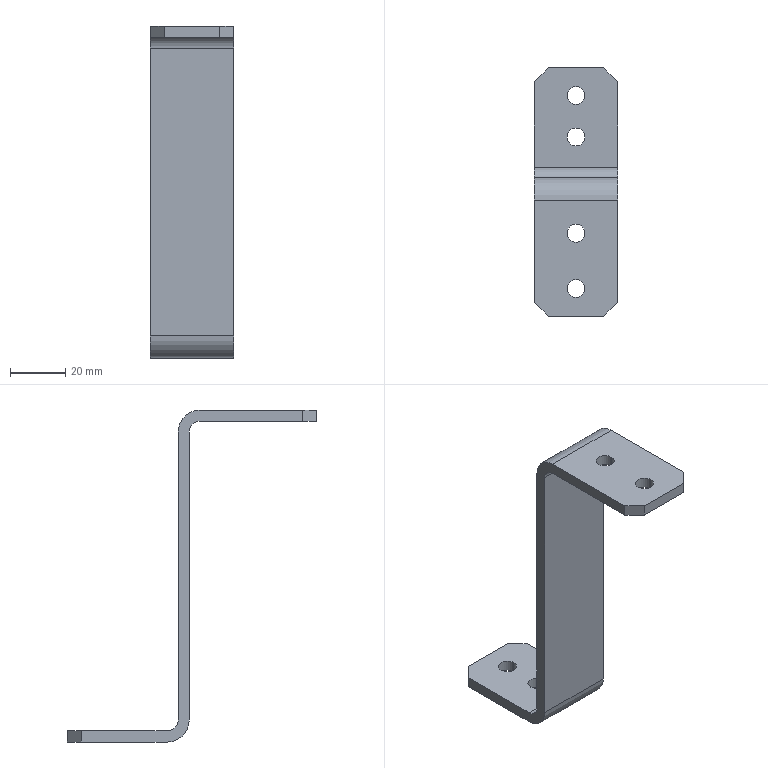Part | SolidWorks | features MBimport 1 | 1 solid | 26 faces | box 30 x 90 x 120 mm | volume 23371 mm3 | plane 14 | cylinder 12 | commonest cylinder face diameters 6.5 x8 8 x2 16 x2
STEP:
#1=CARTESIAN_POINT('',(0.,85.,-109.867));
#2=VERTEX_POINT('',#1);
#3=CARTESIAN_POINT('',(5.,90.,-109.867));
#4=VERTEX_POINT('',#3);
#5=CARTESIAN_POINT('',(5.,90.,-109.867));
#6=DIRECTION('',(0.7071,0.7071,0.));
#7=VECTOR('',#6,1000.);
#8=LINE('',#5,#7);
#9=EDGE_CURVE('',#2,#4,#8,.T.);
#10=ORIENTED_EDGE('',*,*,#9,.F.);
#11=CARTESIAN_POINT('',(0.,85.,-105.867));
#12=VERTEX_POINT('',#11);
#13=CARTESIAN_POINT('',(0.,85.,-109.867));
#14=DIRECTION('',(0.,0.,-1.));
#15=VECTOR('',#14,1000.);
#16=LINE('',#13,#15);
#17=EDGE_CURVE('',#12,#2,#16,.T.);
#18=ORIENTED_EDGE('',*,*,#17,.F.);
#19=CARTESIAN_POINT('',(5.,90.,-105.867));
#20=VERTEX_POINT('',#19);
#21=CARTESIAN_POINT('',(5.,90.,-105.867));
#22=DIRECTION('',(-0.7071,-0.7071,0.));
#23=VECTOR('',#22,1000.);
#24=LINE('',#21,#23);
#25=EDGE_CURVE('',#20,#12,#24,.T.);
#26=ORIENTED_EDGE('',*,*,#25,.F.);
#27=CARTESIAN_POINT('',(5.,90.,-105.867));
#28=DIRECTION('',(0.,0.,1.));
#29=VECTOR('',#28,1000.);
#30=LINE('',#27,#29);
#31=EDGE_CURVE('',#4,#20,#30,.T.);
#32=ORIENTED_EDGE('',*,*,#31,.F.);
#33=EDGE_LOOP('',(#10,#18,#26,#32));
#34=FACE_OUTER_BOUND('',#33,.T.);
#35=CARTESIAN_POINT('',(5.,90.,-105.867));
#36=DIRECTION('',(-0.7071,0.7071,0.));
#37=DIRECTION('',(0.,0.,1.));
#38=AXIS2_PLACEMENT_3D('',#35,#36,#37);
#39=PLANE('',#38);
#40=ADVANCED_FACE('',(#34),#39,.T.);
#41=CARTESIAN_POINT('',(25.,90.,-109.867));
#42=VERTEX_POINT('',#41);
#43=CARTESIAN_POINT('',(30.,85.,-109.867));
#44=VERTEX_POINT('',#43);
#45=CARTESIAN_POINT('',(30.,85.,-109.867));
#46=DIRECTION('',(0.7071,-0.7071,0.));
#47=VECTOR('',#46,1000.);
#48=LINE('',#45,#47);
#49=EDGE_CURVE('',#42,#44,#48,.T.);
#50=ORIENTED_EDGE('',*,*,#49,.F.);
#51=CARTESIAN_POINT('',(25.,90.,-105.867));
#52=VERTEX_POINT('',#51);
#53=CARTESIAN_POINT('',(25.,90.,-105.867));
#54=DIRECTION('',(0.,0.,-1.));
#55=VECTOR('',#54,1000.);
#56=LINE('',#53,#55);
#57=EDGE_CURVE('',#52,#42,#56,.T.);
#58=ORIENTED_EDGE('',*,*,#57,.F.);
#59=CARTESIAN_POINT('',(30.,85.,-105.867));
#60=VERTEX_POINT('',#59);
#61=CARTESIAN_POINT('',(30.,85.,-105.867));
#62=DIRECTION('',(-0.7071,0.7071,0.));
#63=VECTOR('',#62,1000.);
#64=LINE('',#61,#63);
#65=EDGE_CURVE('',#60,#52,#64,.T.);
#66=ORIENTED_EDGE('',*,*,#65,.F.);
#67=CARTESIAN_POINT('',(30.,85.,2.133));
#68=DIRECTION('',(0.,0.,1.));
#69=VECTOR('',#68,1000.);
#70=LINE('',#67,#69);
#71=EDGE_CURVE('',#44,#60,#70,.T.);
#72=ORIENTED_EDGE('',*,*,#71,.F.);
#73=EDGE_LOOP('',(#50,#58,#66,#72));
#74=FACE_OUTER_BOUND('',#73,.T.);
#75=CARTESIAN_POINT('',(30.,85.,2.133));
#76=DIRECTION('',(-0.7071,-0.7071,0.));
#77=DIRECTION('',(-0.7071,0.7071,0.));
#78=AXIS2_PLACEMENT_3D('',#75,#76,#77);
#79=PLANE('',#78);
#80=ADVANCED_FACE('',(#74),#79,.F.);
#81=CARTESIAN_POINT('',(25.,0.,10.133));
#82=VERTEX_POINT('',#81);
#83=CARTESIAN_POINT('',(30.,5.,10.133));
#84=VERTEX_POINT('',#83);
#85=CARTESIAN_POINT('',(30.,5.,10.133));
#86=DIRECTION('',(0.7071,0.7071,0.));
#87=VECTOR('',#86,1000.);
#88=LINE('',#85,#87);
#89=EDGE_CURVE('',#82,#84,#88,.T.);
#90=ORIENTED_EDGE('',*,*,#89,.F.);
#91=CARTESIAN_POINT('',(25.,0.,6.133));
#92=VERTEX_POINT('',#91);
#93=CARTESIAN_POINT('',(25.,0.,6.133));
#94=DIRECTION('',(0.,0.,1.));
#95=VECTOR('',#94,1000.);
#96=LINE('',#93,#95);
#97=EDGE_CURVE('',#92,#82,#96,.T.);
#98=ORIENTED_EDGE('',*,*,#97,.F.);
#99=CARTESIAN_POINT('',(30.,5.,6.133));
#100=VERTEX_POINT('',#99);
#101=CARTESIAN_POINT('',(30.,5.,6.133));
#102=DIRECTION('',(-0.7071,-0.7071,0.));
#103=VECTOR('',#102,1000.);
#104=LINE('',#101,#103);
#105=EDGE_CURVE('',#100,#92,#104,.T.);
#106=ORIENTED_EDGE('',*,*,#105,.F.);
#107=CARTESIAN_POINT('',(30.,5.,2.133));
#108=DIRECTION('',(0.,0.,-1.));
#109=VECTOR('',#108,1000.);
#110=LINE('',#107,#109);
#111=EDGE_CURVE('',#84,#100,#110,.T.);
#112=ORIENTED_EDGE('',*,*,#111,.F.);
#113=EDGE_LOOP('',(#90,#98,#106,#112));
#114=FACE_OUTER_BOUND('',#113,.T.);
#115=CARTESIAN_POINT('',(30.,5.,2.133));
#116=DIRECTION('',(-0.7071,0.7071,0.));
#117=DIRECTION('',(0.,0.,1.));
#118=AXIS2_PLACEMENT_3D('',#115,#116,#117);
#119=PLANE('',#118);
#120=ADVANCED_FACE('',(#114),#119,.F.);
#121=CARTESIAN_POINT('',(0.,5.,10.133));
#122=VERTEX_POINT('',#121);
#123=CARTESIAN_POINT('',(5.,0.,10.133));
#124=VERTEX_POINT('',#123);
#125=CARTESIAN_POINT('',(5.,0.,10.133));
#126=DIRECTION('',(0.7071,-0.7071,0.));
#127=VECTOR('',#126,1000.);
#128=LINE('',#125,#127);
#129=EDGE_CURVE('',#122,#124,#128,.T.);
#130=ORIENTED_EDGE('',*,*,#129,.F.);
#131=CARTESIAN_POINT('',(0.,5.,6.133));
#132=VERTEX_POINT('',#131);
#133=CARTESIAN_POINT('',(0.,5.,10.133));
#134=DIRECTION('',(0.,0.,1.));
#135=VECTOR('',#134,1000.);
#136=LINE('',#133,#135);
#137=EDGE_CURVE('',#132,#122,#136,.T.);
#138=ORIENTED_EDGE('',*,*,#137,.F.);
#139=CARTESIAN_POINT('',(5.,0.,6.133));
#140=VERTEX_POINT('',#139);
#141=CARTESIAN_POINT('',(5.,0.,6.133));
#142=DIRECTION('',(-0.7071,0.7071,0.));
#143=VECTOR('',#142,1000.);
#144=LINE('',#141,#143);
#145=EDGE_CURVE('',#140,#132,#144,.T.);
#146=ORIENTED_EDGE('',*,*,#145,.F.);
#147=CARTESIAN_POINT('',(5.,0.,6.133));
#148=DIRECTION('',(0.,0.,-1.));
#149=VECTOR('',#148,1000.);
#150=LINE('',#147,#149);
#151=EDGE_CURVE('',#124,#140,#150,.T.);
#152=ORIENTED_EDGE('',*,*,#151,.F.);
#153=EDGE_LOOP('',(#130,#138,#146,#152));
#154=FACE_OUTER_BOUND('',#153,.T.);
#155=CARTESIAN_POINT('',(5.,0.,6.133));
#156=DIRECTION('',(-0.7071,-0.7071,0.));
#157=DIRECTION('',(-0.7071,0.7071,0.));
#158=AXIS2_PLACEMENT_3D('',#155,#156,#157);
#159=PLANE('',#158);
#160=ADVANCED_FACE('',(#154),#159,.T.);
#161=CARTESIAN_POINT('',(11.75,30.,6.133));
#162=VERTEX_POINT('',#161);
#163=CARTESIAN_POINT('',(11.75,30.,10.133));
#164=VERTEX_POINT('',#163);
#165=CARTESIAN_POINT('',(11.75,30.,-19.867));
#166=DIRECTION('',(0.,0.,1.));
#167=VECTOR('',#166,1000.);
#168=LINE('',#165,#167);
#169=EDGE_CURVE('',#162,#164,#168,.T.);
#170=ORIENTED_EDGE('',*,*,#169,.F.);
#171=CARTESIAN_POINT('',(18.25,30.,6.133));
#172=VERTEX_POINT('',#171);
#173=CARTESIAN_POINT('',(15.,30.,6.133));
#174=DIRECTION('',(0.,0.,1.));
#175=DIRECTION('',(0.,-1.,0.));
#176=AXIS2_PLACEMENT_3D('',#173,#174,#175);
#177=CIRCLE('',#176,3.25);
#178=EDGE_CURVE('',#172,#162,#177,.T.);
#179=ORIENTED_EDGE('',*,*,#178,.F.);
#180=CARTESIAN_POINT('',(18.25,30.,10.133));
#181=VERTEX_POINT('',#180);
#182=CARTESIAN_POINT('',(18.25,30.,-19.867));
#183=DIRECTION('',(0.,0.,1.));
#184=VECTOR('',#183,1000.);
#185=LINE('',#182,#184);
#186=EDGE_CURVE('',#172,#181,#185,.T.);
#187=ORIENTED_EDGE('',*,*,#186,.T.);
#188=CARTESIAN_POINT('',(15.,30.,10.133));
#189=DIRECTION('',(0.,0.,1.));
#190=DIRECTION('',(1.,0.,0.));
#191=AXIS2_PLACEMENT_3D('',#188,#189,#190);
#192=CIRCLE('',#191,3.25);
#193=EDGE_CURVE('',#181,#164,#192,.T.);
#194=ORIENTED_EDGE('',*,*,#193,.T.);
#195=EDGE_LOOP('',(#170,#179,#187,#194));
#196=FACE_OUTER_BOUND('',#195,.T.);
#197=CARTESIAN_POINT('',(15.,30.,-19.867));
#198=DIRECTION('',(0.,0.,1.));
#199=DIRECTION('',(1.,0.,0.));
#200=AXIS2_PLACEMENT_3D('',#197,#198,#199);
#201=CYLINDRICAL_SURFACE('',#200,3.25);
#202=ADVANCED_FACE('',(#196),#201,.F.);
#203=CARTESIAN_POINT('',(11.75,10.,6.133));
#204=VERTEX_POINT('',#203);
#205=CARTESIAN_POINT('',(11.75,10.,10.133));
#206=VERTEX_POINT('',#205);
#207=CARTESIAN_POINT('',(11.75,10.,-19.867));
#208=DIRECTION('',(0.,0.,1.));
#209=VECTOR('',#208,1000.);
#210=LINE('',#207,#209);
#211=EDGE_CURVE('',#204,#206,#210,.T.);
#212=ORIENTED_EDGE('',*,*,#211,.F.);
#213=CARTESIAN_POINT('',(18.25,10.,6.133));
#214=VERTEX_POINT('',#213);
#215=CARTESIAN_POINT('',(15.,10.,6.133));
#216=DIRECTION('',(0.,0.,1.));
#217=DIRECTION('',(0.,-1.,0.));
#218=AXIS2_PLACEMENT_3D('',#215,#216,#217);
#219=CIRCLE('',#218,3.25);
#220=EDGE_CURVE('',#214,#204,#219,.T.);
#221=ORIENTED_EDGE('',*,*,#220,.F.);
#222=CARTESIAN_POINT('',(18.25,10.,10.133));
#223=VERTEX_POINT('',#222);
#224=CARTESIAN_POINT('',(18.25,10.,-19.867));
#225=DIRECTION('',(0.,0.,1.));
#226=VECTOR('',#225,1000.);
#227=LINE('',#224,#226);
#228=EDGE_CURVE('',#214,#223,#227,.T.);
#229=ORIENTED_EDGE('',*,*,#228,.T.);
#230=CARTESIAN_POINT('',(15.,10.,10.133));
#231=DIRECTION('',(0.,0.,1.));
#232=DIRECTION('',(1.,0.,0.));
#233=AXIS2_PLACEMENT_3D('',#230,#231,#232);
#234=CIRCLE('',#233,3.25);
#235=EDGE_CURVE('',#223,#206,#234,.T.);
#236=ORIENTED_EDGE('',*,*,#235,.T.);
#237=EDGE_LOOP('',(#212,#221,#229,#236));
#238=FACE_OUTER_BOUND('',#237,.T.);
#239=CARTESIAN_POINT('',(15.,10.,-19.867));
#240=DIRECTION('',(0.,0.,1.));
#241=DIRECTION('',(1.,0.,0.));
#242=AXIS2_PLACEMENT_3D('',#239,#240,#241);
#243=CYLINDRICAL_SURFACE('',#242,3.25);
#244=ADVANCED_FACE('',(#238),#243,.F.);
#245=CARTESIAN_POINT('',(11.75,80.,-109.867));
#246=VERTEX_POINT('',#245);
#247=CARTESIAN_POINT('',(11.75,80.,-105.867));
#248=VERTEX_POINT('',#247);
#249=CARTESIAN_POINT('',(11.75,80.,-135.867));
#250=DIRECTION('',(0.,0.,1.));
#251=VECTOR('',#250,1000.);
#252=LINE('',#249,#251);
#253=EDGE_CURVE('',#246,#248,#252,.T.);
#254=ORIENTED_EDGE('',*,*,#253,.F.);
#255=CARTESIAN_POINT('',(18.25,80.,-109.867));
#256=VERTEX_POINT('',#255);
#257=CARTESIAN_POINT('',(15.,80.,-109.867));
#258=DIRECTION('',(0.,0.,1.));
#259=DIRECTION('',(0.,-1.,0.));
#260=AXIS2_PLACEMENT_3D('',#257,#258,#259);
#261=CIRCLE('',#260,3.25);
#262=EDGE_CURVE('',#256,#246,#261,.T.);
#263=ORIENTED_EDGE('',*,*,#262,.F.);
#264=CARTESIAN_POINT('',(18.25,80.,-105.867));
#265=VERTEX_POINT('',#264);
#266=CARTESIAN_POINT('',(18.25,80.,-135.867));
#267=DIRECTION('',(0.,0.,1.));
#268=VECTOR('',#267,1000.);
#269=LINE('',#266,#268);
#270=EDGE_CURVE('',#256,#265,#269,.T.);
#271=ORIENTED_EDGE('',*,*,#270,.T.);
#272=CARTESIAN_POINT('',(15.,80.,-105.867));
#273=DIRECTION('',(0.,0.,1.));
#274=DIRECTION('',(1.,0.,0.));
#275=AXIS2_PLACEMENT_3D('',#272,#273,#274);
#276=CIRCLE('',#275,3.25);
#277=EDGE_CURVE('',#265,#248,#276,.T.);
#278=ORIENTED_EDGE('',*,*,#277,.T.);
#279=EDGE_LOOP('',(#254,#263,#271,#278));
#280=FACE_OUTER_BOUND('',#279,.T.);
#281=CARTESIAN_POINT('',(15.,80.,-135.867));
#282=DIRECTION('',(0.,0.,1.));
#283=DIRECTION('',(1.,0.,0.));
#284=AXIS2_PLACEMENT_3D('',#281,#282,#283);
#285=CYLINDRICAL_SURFACE('',#284,3.25);
#286=ADVANCED_FACE('',(#280),#285,.F.);
#287=CARTESIAN_POINT('',(11.75,65.,-109.867));
#288=VERTEX_POINT('',#287);
#289=CARTESIAN_POINT('',(11.75,65.,-105.867));
#290=VERTEX_POINT('',#289);
#291=CARTESIAN_POINT('',(11.75,65.,-135.867));
#292=DIRECTION('',(0.,0.,1.));
#293=VECTOR('',#292,1000.);
#294=LINE('',#291,#293);
#295=EDGE_CURVE('',#288,#290,#294,.T.);
#296=ORIENTED_EDGE('',*,*,#295,.F.);
#297=CARTESIAN_POINT('',(18.25,65.,-109.867));
#298=VERTEX_POINT('',#297);
#299=CARTESIAN_POINT('',(15.,65.,-109.867));
#300=DIRECTION('',(0.,0.,1.));
#301=DIRECTION('',(0.,-1.,0.));
#302=AXIS2_PLACEMENT_3D('',#299,#300,#301);
#303=CIRCLE('',#302,3.25);
#304=EDGE_CURVE('',#298,#288,#303,.T.);
#305=ORIENTED_EDGE('',*,*,#304,.F.);
#306=CARTESIAN_POINT('',(18.25,65.,-105.867));
#307=VERTEX_POINT('',#306);
#308=CARTESIAN_POINT('',(18.25,65.,-135.867));
#309=DIRECTION('',(0.,0.,1.));
#310=VECTOR('',#309,1000.);
#311=LINE('',#308,#310);
#312=EDGE_CURVE('',#298,#307,#311,.T.);
#313=ORIENTED_EDGE('',*,*,#312,.T.);
#314=CARTESIAN_POINT('',(15.,65.,-105.867));
#315=DIRECTION('',(0.,0.,1.));
#316=DIRECTION('',(1.,0.,0.));
#317=AXIS2_PLACEMENT_3D('',#314,#315,#316);
#318=CIRCLE('',#317,3.25);
#319=EDGE_CURVE('',#307,#290,#318,.T.);
#320=ORIENTED_EDGE('',*,*,#319,.T.);
#321=EDGE_LOOP('',(#296,#305,#313,#320));
#322=FACE_OUTER_BOUND('',#321,.T.);
#323=CARTESIAN_POINT('',(15.,65.,-135.867));
#324=DIRECTION('',(0.,0.,1.));
#325=DIRECTION('',(1.,0.,0.));
#326=AXIS2_PLACEMENT_3D('',#323,#324,#325);
#327=CYLINDRICAL_SURFACE('',#326,3.25);
#328=ADVANCED_FACE('',(#322),#327,.F.);
#329=CARTESIAN_POINT('',(0.,42.,6.133));
#330=VERTEX_POINT('',#329);
#331=CARTESIAN_POINT('',(0.,42.,6.133));
#332=DIRECTION('',(0.,1.,0.));
#333=VECTOR('',#332,1000.);
#334=LINE('',#331,#333);
#335=EDGE_CURVE('',#132,#330,#334,.T.);
#336=ORIENTED_EDGE('',*,*,#335,.F.);
#337=ORIENTED_EDGE('',*,*,#137,.T.);
#338=CARTESIAN_POINT('',(0.,42.,10.133));
#339=VERTEX_POINT('',#338);
#340=CARTESIAN_POINT('',(0.,0.,10.133));
#341=DIRECTION('',(0.,-1.,0.));
#342=VECTOR('',#341,1000.);
#343=LINE('',#340,#342);
#344=EDGE_CURVE('',#339,#122,#343,.T.);
#345=ORIENTED_EDGE('',*,*,#344,.F.);
#346=CARTESIAN_POINT('',(0.,50.,2.133));
#347=VERTEX_POINT('',#346);
#348=CARTESIAN_POINT('',(0.,42.,2.133));
#349=DIRECTION('',(1.,0.,0.));
#350=DIRECTION('',(0.,0.,1.));
#351=AXIS2_PLACEMENT_3D('',#348,#349,#350);
#352=CIRCLE('',#351,8.);
#353=EDGE_CURVE('',#347,#339,#352,.T.);
#354=ORIENTED_EDGE('',*,*,#353,.F.);
#355=CARTESIAN_POINT('',(0.,50.,-101.867));
#356=VERTEX_POINT('',#355);
#357=CARTESIAN_POINT('',(0.,50.,2.133));
#358=DIRECTION('',(0.,0.,1.));
#359=VECTOR('',#358,1000.);
#360=LINE('',#357,#359);
#361=EDGE_CURVE('',#356,#347,#360,.T.);
#362=ORIENTED_EDGE('',*,*,#361,.F.);
#363=CARTESIAN_POINT('',(0.,54.,-105.867));
#364=VERTEX_POINT('',#363);
#365=CARTESIAN_POINT('',(0.,54.,-101.867));
#366=DIRECTION('',(-1.,0.,0.));
#367=DIRECTION('',(0.,0.,-1.));
#368=AXIS2_PLACEMENT_3D('',#365,#366,#367);
#369=CIRCLE('',#368,4.);
#370=EDGE_CURVE('',#364,#356,#369,.T.);
#371=ORIENTED_EDGE('',*,*,#370,.F.);
#372=CARTESIAN_POINT('',(0.,54.,-105.867));
#373=DIRECTION('',(0.,-1.,0.));
#374=VECTOR('',#373,1000.);
#375=LINE('',#372,#374);
#376=EDGE_CURVE('',#12,#364,#375,.T.);
#377=ORIENTED_EDGE('',*,*,#376,.F.);
#378=ORIENTED_EDGE('',*,*,#17,.T.);
#379=CARTESIAN_POINT('',(0.,54.,-109.867));
#380=VERTEX_POINT('',#379);
#381=CARTESIAN_POINT('',(0.,90.,-109.867));
#382=DIRECTION('',(0.,1.,0.));
#383=VECTOR('',#382,1000.);
#384=LINE('',#381,#383);
#385=EDGE_CURVE('',#380,#2,#384,.T.);
#386=ORIENTED_EDGE('',*,*,#385,.F.);
#387=CARTESIAN_POINT('',(0.,46.,-101.867));
#388=VERTEX_POINT('',#387);
#389=CARTESIAN_POINT('',(0.,54.,-101.867));
#390=DIRECTION('',(1.,0.,0.));
#391=DIRECTION('',(0.,0.,-1.));
#392=AXIS2_PLACEMENT_3D('',#389,#390,#391);
#393=CIRCLE('',#392,8.);
#394=EDGE_CURVE('',#388,#380,#393,.T.);
#395=ORIENTED_EDGE('',*,*,#394,.F.);
#396=CARTESIAN_POINT('',(0.,46.,2.133));
#397=VERTEX_POINT('',#396);
#398=CARTESIAN_POINT('',(0.,46.,-101.867));
#399=DIRECTION('',(0.,0.,-1.));
#400=VECTOR('',#399,1000.);
#401=LINE('',#398,#400);
#402=EDGE_CURVE('',#397,#388,#401,.T.);
#403=ORIENTED_EDGE('',*,*,#402,.F.);
#404=CARTESIAN_POINT('',(0.,42.,2.133));
#405=DIRECTION('',(-1.,0.,0.));
#406=DIRECTION('',(0.,0.,1.));
#407=AXIS2_PLACEMENT_3D('',#404,#405,#406);
#408=CIRCLE('',#407,4.);
#409=EDGE_CURVE('',#330,#397,#408,.T.);
#410=ORIENTED_EDGE('',*,*,#409,.F.);
#411=EDGE_LOOP('',(#336,#337,#345,#354,#362,#371,#377,#378,#386,#395,#403,#410));
#412=FACE_OUTER_BOUND('',#411,.T.);
#413=CARTESIAN_POINT('',(0.,42.,2.133));
#414=DIRECTION('',(-1.,0.,0.));
#415=DIRECTION('',(0.,0.,1.));
#416=AXIS2_PLACEMENT_3D('',#413,#414,#415);
#417=PLANE('',#416);
#418=ADVANCED_FACE('',(#412),#417,.T.);
#419=CARTESIAN_POINT('',(30.,42.,10.133));
#420=VERTEX_POINT('',#419);
#421=CARTESIAN_POINT('',(30.,0.,10.133));
#422=DIRECTION('',(0.,-1.,0.));
#423=VECTOR('',#422,1000.);
#424=LINE('',#421,#423);
#425=EDGE_CURVE('',#420,#84,#424,.T.);
#426=ORIENTED_EDGE('',*,*,#425,.T.);
#427=ORIENTED_EDGE('',*,*,#111,.T.);
#428=CARTESIAN_POINT('',(30.,42.,6.133));
#429=VERTEX_POINT('',#428);
#430=CARTESIAN_POINT('',(30.,42.,6.133));
#431=DIRECTION('',(0.,1.,0.));
#432=VECTOR('',#431,1000.);
#433=LINE('',#430,#432);
#434=EDGE_CURVE('',#100,#429,#433,.T.);
#435=ORIENTED_EDGE('',*,*,#434,.T.);
#436=CARTESIAN_POINT('',(30.,46.,2.133));
#437=VERTEX_POINT('',#436);
#438=CARTESIAN_POINT('',(30.,42.,2.133));
#439=DIRECTION('',(-1.,0.,0.));
#440=DIRECTION('',(0.,0.,1.));
#441=AXIS2_PLACEMENT_3D('',#438,#439,#440);
#442=CIRCLE('',#441,4.);
#443=EDGE_CURVE('',#429,#437,#442,.T.);
#444=ORIENTED_EDGE('',*,*,#443,.T.);
#445=CARTESIAN_POINT('',(30.,46.,-101.867));
#446=VERTEX_POINT('',#445);
#447=CARTESIAN_POINT('',(30.,46.,-101.867));
#448=DIRECTION('',(0.,0.,-1.));
#449=VECTOR('',#448,1000.);
#450=LINE('',#447,#449);
#451=EDGE_CURVE('',#437,#446,#450,.T.);
#452=ORIENTED_EDGE('',*,*,#451,.T.);
#453=CARTESIAN_POINT('',(30.,54.,-109.867));
#454=VERTEX_POINT('',#453);
#455=CARTESIAN_POINT('',(30.,54.,-101.867));
#456=DIRECTION('',(1.,0.,0.));
#457=DIRECTION('',(0.,0.,-1.));
#458=AXIS2_PLACEMENT_3D('',#455,#456,#457);
#459=CIRCLE('',#458,8.);
#460=EDGE_CURVE('',#446,#454,#459,.T.);
#461=ORIENTED_EDGE('',*,*,#460,.T.);
#462=CARTESIAN_POINT('',(30.,90.,-109.867));
#463=DIRECTION('',(0.,1.,0.));
#464=VECTOR('',#463,1000.);
#465=LINE('',#462,#464);
#466=EDGE_CURVE('',#454,#44,#465,.T.);
#467=ORIENTED_EDGE('',*,*,#466,.T.);
#468=ORIENTED_EDGE('',*,*,#71,.T.);
#469=CARTESIAN_POINT('',(30.,54.,-105.867));
#470=VERTEX_POINT('',#469);
#471=CARTESIAN_POINT('',(30.,54.,-105.867));
#472=DIRECTION('',(0.,-1.,0.));
#473=VECTOR('',#472,1000.);
#474=LINE('',#471,#473);
#475=EDGE_CURVE('',#60,#470,#474,.T.);
#476=ORIENTED_EDGE('',*,*,#475,.T.);
#477=CARTESIAN_POINT('',(30.,50.,-101.867));
#478=VERTEX_POINT('',#477);
#479=CARTESIAN_POINT('',(30.,54.,-101.867));
#480=DIRECTION('',(-1.,0.,0.));
#481=DIRECTION('',(0.,0.,-1.));
#482=AXIS2_PLACEMENT_3D('',#479,#480,#481);
#483=CIRCLE('',#482,4.);
#484=EDGE_CURVE('',#470,#478,#483,.T.);
#485=ORIENTED_EDGE('',*,*,#484,.T.);
#486=CARTESIAN_POINT('',(30.,50.,2.133));
#487=VERTEX_POINT('',#486);
#488=CARTESIAN_POINT('',(30.,50.,2.133));
#489=DIRECTION('',(0.,0.,1.));
#490=VECTOR('',#489,1000.);
#491=LINE('',#488,#490);
#492=EDGE_CURVE('',#478,#487,#491,.T.);
#493=ORIENTED_EDGE('',*,*,#492,.T.);
#494=CARTESIAN_POINT('',(30.,42.,2.133));
#495=DIRECTION('',(1.,0.,0.));
#496=DIRECTION('',(0.,0.,1.));
#497=AXIS2_PLACEMENT_3D('',#494,#495,#496);
#498=CIRCLE('',#497,8.);
#499=EDGE_CURVE('',#487,#420,#498,.T.);
#500=ORIENTED_EDGE('',*,*,#499,.T.);
#501=EDGE_LOOP('',(#426,#427,#435,#444,#452,#461,#467,#468,#476,#485,#493,#500));
#502=FACE_OUTER_BOUND('',#501,.T.);
#503=CARTESIAN_POINT('',(30.,42.,2.133));
#504=DIRECTION('',(-1.,0.,0.));
#505=DIRECTION('',(0.,0.,1.));
#506=AXIS2_PLACEMENT_3D('',#503,#504,#505);
#507=PLANE('',#506);
#508=ADVANCED_FACE('',(#502),#507,.F.);
#509=CARTESIAN_POINT('',(30.,0.,10.133));
#510=DIRECTION('',(-1.,0.,0.));
#511=VECTOR('',#510,1000.);
#512=LINE('',#509,#511);
#513=EDGE_CURVE('',#82,#124,#512,.T.);
#514=ORIENTED_EDGE('',*,*,#513,.T.);
#515=ORIENTED_EDGE('',*,*,#151,.T.);
#516=CARTESIAN_POINT('',(30.,0.,6.133));
#517=DIRECTION('',(-1.,0.,0.));
#518=VECTOR('',#517,1000.);
#519=LINE('',#516,#518);
#520=EDGE_CURVE('',#92,#140,#519,.T.);
#521=ORIENTED_EDGE('',*,*,#520,.F.);
#522=ORIENTED_EDGE('',*,*,#97,.T.);
#523=EDGE_LOOP('',(#514,#515,#521,#522));
#524=FACE_OUTER_BOUND('',#523,.T.);
#525=CARTESIAN_POINT('',(30.,0.,6.133));
#526=DIRECTION('',(0.,1.,0.));
#527=DIRECTION('',(1.,0.,0.));
#528=AXIS2_PLACEMENT_3D('',#525,#526,#527);
#529=PLANE('',#528);
#530=ADVANCED_FACE('',(#524),#529,.F.);
#531=ORIENTED_EDGE('',*,*,#235,.F.);
#532=CARTESIAN_POINT('',(15.,10.,10.133));
#533=DIRECTION('',(0.,0.,1.));
#534=DIRECTION('',(1.,0.,0.));
#535=AXIS2_PLACEMENT_3D('',#532,#533,#534);
#536=CIRCLE('',#535,3.25);
#537=EDGE_CURVE('',#206,#223,#536,.T.);
#538=ORIENTED_EDGE('',*,*,#537,.F.);
#539=EDGE_LOOP('',(#531,#538));
#540=FACE_BOUND('',#539,.T.);
#541=ORIENTED_EDGE('',*,*,#193,.F.);
#542=CARTESIAN_POINT('',(15.,30.,10.133));
#543=DIRECTION('',(0.,0.,1.));
#544=DIRECTION('',(1.,0.,0.));
#545=AXIS2_PLACEMENT_3D('',#542,#543,#544);
#546=CIRCLE('',#545,3.25);
#547=EDGE_CURVE('',#164,#181,#546,.T.);
#548=ORIENTED_EDGE('',*,*,#547,.F.);
#549=EDGE_LOOP('',(#541,#548));
#550=FACE_BOUND('',#549,.T.);
#551=ORIENTED_EDGE('',*,*,#344,.T.);
#552=ORIENTED_EDGE('',*,*,#129,.T.);
#553=ORIENTED_EDGE('',*,*,#513,.F.);
#554=ORIENTED_EDGE('',*,*,#89,.T.);
#555=ORIENTED_EDGE('',*,*,#425,.F.);
#556=CARTESIAN_POINT('',(30.,42.,10.133));
#557=DIRECTION('',(-1.,0.,0.));
#558=VECTOR('',#557,1000.);
#559=LINE('',#556,#558);
#560=EDGE_CURVE('',#420,#339,#559,.T.);
#561=ORIENTED_EDGE('',*,*,#560,.T.);
#562=EDGE_LOOP('',(#551,#552,#553,#554,#555,#561));
#563=FACE_OUTER_BOUND('',#562,.T.);
#564=CARTESIAN_POINT('',(30.,0.,10.133));
#565=DIRECTION('',(0.,0.,-1.));
#566=DIRECTION('',(0.,-1.,0.));
#567=AXIS2_PLACEMENT_3D('',#564,#565,#566);
#568=PLANE('',#567);
#569=ADVANCED_FACE('',(#540,#550,#563),#568,.F.);
#570=ORIENTED_EDGE('',*,*,#353,.T.);
#571=ORIENTED_EDGE('',*,*,#560,.F.);
#572=ORIENTED_EDGE('',*,*,#499,.F.);
#573=CARTESIAN_POINT('',(30.,50.,2.133));
#574=DIRECTION('',(-1.,0.,0.));
#575=VECTOR('',#574,1000.);
#576=LINE('',#573,#575);
#577=EDGE_CURVE('',#487,#347,#576,.T.);
#578=ORIENTED_EDGE('',*,*,#577,.T.);
#579=EDGE_LOOP('',(#570,#571,#572,#578));
#580=FACE_OUTER_BOUND('',#579,.T.);
#581=CARTESIAN_POINT('',(30.,42.,2.133));
#582=DIRECTION('',(-1.,0.,0.));
#583=DIRECTION('',(0.,0.,1.));
#584=AXIS2_PLACEMENT_3D('',#581,#582,#583);
#585=CYLINDRICAL_SURFACE('',#584,8.);
#586=ADVANCED_FACE('',(#580),#585,.T.);
#587=ORIENTED_EDGE('',*,*,#361,.T.);
#588=ORIENTED_EDGE('',*,*,#577,.F.);
#589=ORIENTED_EDGE('',*,*,#492,.F.);
#590=CARTESIAN_POINT('',(30.,50.,-101.867));
#591=DIRECTION('',(-1.,0.,0.));
#592=VECTOR('',#591,1000.);
#593=LINE('',#590,#592);
#594=EDGE_CURVE('',#478,#356,#593,.T.);
#595=ORIENTED_EDGE('',*,*,#594,.T.);
#596=EDGE_LOOP('',(#587,#588,#589,#595));
#597=FACE_OUTER_BOUND('',#596,.T.);
#598=CARTESIAN_POINT('',(30.,50.,2.133));
#599=DIRECTION('',(0.,-1.,0.));
#600=DIRECTION('',(0.,0.,-1.));
#601=AXIS2_PLACEMENT_3D('',#598,#599,#600);
#602=PLANE('',#601);
#603=ADVANCED_FACE('',(#597),#602,.F.);
#604=ORIENTED_EDGE('',*,*,#370,.T.);
#605=ORIENTED_EDGE('',*,*,#594,.F.);
#606=ORIENTED_EDGE('',*,*,#484,.F.);
#607=CARTESIAN_POINT('',(30.,54.,-105.867));
#608=DIRECTION('',(-1.,0.,0.));
#609=VECTOR('',#608,1000.);
#610=LINE('',#607,#609);
#611=EDGE_CURVE('',#470,#364,#610,.T.);
#612=ORIENTED_EDGE('',*,*,#611,.T.);
#613=EDGE_LOOP('',(#604,#605,#606,#612));
#614=FACE_OUTER_BOUND('',#613,.T.);
#615=CARTESIAN_POINT('',(30.,54.,-101.867));
#616=DIRECTION('',(-1.,0.,0.));
#617=DIRECTION('',(0.,0.,1.));
#618=AXIS2_PLACEMENT_3D('',#615,#616,#617);
#619=CYLINDRICAL_SURFACE('',#618,4.);
#620=ADVANCED_FACE('',(#614),#619,.F.);
#621=ORIENTED_EDGE('',*,*,#319,.F.);
#622=CARTESIAN_POINT('',(15.,65.,-105.867));
#623=DIRECTION('',(0.,0.,1.));
#624=DIRECTION('',(1.,0.,0.));
#625=AXIS2_PLACEMENT_3D('',#622,#623,#624);
#626=CIRCLE('',#625,3.25);
#627=EDGE_CURVE('',#290,#307,#626,.T.);
#628=ORIENTED_EDGE('',*,*,#627,.F.);
#629=EDGE_LOOP('',(#621,#628));
#630=FACE_BOUND('',#629,.T.);
#631=ORIENTED_EDGE('',*,*,#277,.F.);
#632=CARTESIAN_POINT('',(15.,80.,-105.867));
#633=DIRECTION('',(0.,0.,1.));
#634=DIRECTION('',(1.,0.,0.));
#635=AXIS2_PLACEMENT_3D('',#632,#633,#634);
#636=CIRCLE('',#635,3.25);
#637=EDGE_CURVE('',#248,#265,#636,.T.);
#638=ORIENTED_EDGE('',*,*,#637,.F.);
#639=EDGE_LOOP('',(#631,#638));
#640=FACE_BOUND('',#639,.T.);
#641=ORIENTED_EDGE('',*,*,#475,.F.);
#642=ORIENTED_EDGE('',*,*,#65,.T.);
#643=CARTESIAN_POINT('',(30.,90.,-105.867));
#644=DIRECTION('',(-1.,0.,0.));
#645=VECTOR('',#644,1000.);
#646=LINE('',#643,#645);
#647=EDGE_CURVE('',#52,#20,#646,.T.);
#648=ORIENTED_EDGE('',*,*,#647,.T.);
#649=ORIENTED_EDGE('',*,*,#25,.T.);
#650=ORIENTED_EDGE('',*,*,#376,.T.);
#651=ORIENTED_EDGE('',*,*,#611,.F.);
#652=EDGE_LOOP('',(#641,#642,#648,#649,#650,#651));
#653=FACE_OUTER_BOUND('',#652,.T.);
#654=CARTESIAN_POINT('',(30.,54.,-105.867));
#655=DIRECTION('',(0.,0.,-1.));
#656=DIRECTION('',(0.,-1.,0.));
#657=AXIS2_PLACEMENT_3D('',#654,#655,#656);
#658=PLANE('',#657);
#659=ADVANCED_FACE('',(#630,#640,#653),#658,.F.);
#660=ORIENTED_EDGE('',*,*,#647,.F.);
#661=ORIENTED_EDGE('',*,*,#57,.T.);
#662=CARTESIAN_POINT('',(30.,90.,-109.867));
#663=DIRECTION('',(-1.,0.,0.));
#664=VECTOR('',#663,1000.);
#665=LINE('',#662,#664);
#666=EDGE_CURVE('',#42,#4,#665,.T.);
#667=ORIENTED_EDGE('',*,*,#666,.T.);
#668=ORIENTED_EDGE('',*,*,#31,.T.);
#669=EDGE_LOOP('',(#660,#661,#667,#668));
#670=FACE_OUTER_BOUND('',#669,.T.);
#671=CARTESIAN_POINT('',(30.,90.,-105.867));
#672=DIRECTION('',(0.,-1.,0.));
#673=DIRECTION('',(0.,0.,-1.));
#674=AXIS2_PLACEMENT_3D('',#671,#672,#673);
#675=PLANE('',#674);
#676=ADVANCED_FACE('',(#670),#675,.F.);
#677=ORIENTED_EDGE('',*,*,#304,.T.);
#678=CARTESIAN_POINT('',(15.,65.,-109.867));
#679=DIRECTION('',(0.,0.,1.));
#680=DIRECTION('',(0.,-1.,0.));
#681=AXIS2_PLACEMENT_3D('',#678,#679,#680);
#682=CIRCLE('',#681,3.25);
#683=EDGE_CURVE('',#288,#298,#682,.T.);
#684=ORIENTED_EDGE('',*,*,#683,.T.);
#685=EDGE_LOOP('',(#677,#684));
#686=FACE_BOUND('',#685,.T.);
#687=ORIENTED_EDGE('',*,*,#262,.T.);
#688=CARTESIAN_POINT('',(15.,80.,-109.867));
#689=DIRECTION('',(0.,0.,1.));
#690=DIRECTION('',(0.,-1.,0.));
#691=AXIS2_PLACEMENT_3D('',#688,#689,#690);
#692=CIRCLE('',#691,3.25);
#693=EDGE_CURVE('',#246,#256,#692,.T.);
#694=ORIENTED_EDGE('',*,*,#693,.T.);
#695=EDGE_LOOP('',(#687,#694));
#696=FACE_BOUND('',#695,.T.);
#697=ORIENTED_EDGE('',*,*,#666,.F.);
#698=ORIENTED_EDGE('',*,*,#49,.T.);
#699=ORIENTED_EDGE('',*,*,#466,.F.);
#700=CARTESIAN_POINT('',(30.,54.,-109.867));
#701=DIRECTION('',(-1.,0.,0.));
#702=VECTOR('',#701,1000.);
#703=LINE('',#700,#702);
#704=EDGE_CURVE('',#454,#380,#703,.T.);
#705=ORIENTED_EDGE('',*,*,#704,.T.);
#706=ORIENTED_EDGE('',*,*,#385,.T.);
#707=ORIENTED_EDGE('',*,*,#9,.T.);
#708=EDGE_LOOP('',(#697,#698,#699,#705,#706,#707));
#709=FACE_OUTER_BOUND('',#708,.T.);
#710=CARTESIAN_POINT('',(30.,90.,-109.867));
#711=DIRECTION('',(0.,0.,1.));
#712=DIRECTION('',(0.,-1.,0.));
#713=AXIS2_PLACEMENT_3D('',#710,#711,#712);
#714=PLANE('',#713);
#715=ADVANCED_FACE('',(#686,#696,#709),#714,.F.);
#716=ORIENTED_EDGE('',*,*,#394,.T.);
#717=ORIENTED_EDGE('',*,*,#704,.F.);
#718=ORIENTED_EDGE('',*,*,#460,.F.);
#719=CARTESIAN_POINT('',(30.,46.,-101.867));
#720=DIRECTION('',(-1.,0.,0.));
#721=VECTOR('',#720,1000.);
#722=LINE('',#719,#721);
#723=EDGE_CURVE('',#446,#388,#722,.T.);
#724=ORIENTED_EDGE('',*,*,#723,.T.);
#725=EDGE_LOOP('',(#716,#717,#718,#724));
#726=FACE_OUTER_BOUND('',#725,.T.);
#727=CARTESIAN_POINT('',(30.,54.,-101.867));
#728=DIRECTION('',(-1.,0.,0.));
#729=DIRECTION('',(0.,0.,1.));
#730=AXIS2_PLACEMENT_3D('',#727,#728,#729);
#731=CYLINDRICAL_SURFACE('',#730,8.);
#732=ADVANCED_FACE('',(#726),#731,.T.);
#733=ORIENTED_EDGE('',*,*,#402,.T.);
#734=ORIENTED_EDGE('',*,*,#723,.F.);
#735=ORIENTED_EDGE('',*,*,#451,.F.);
#736=CARTESIAN_POINT('',(30.,46.,2.133));
#737=DIRECTION('',(-1.,0.,0.));
#738=VECTOR('',#737,1000.);
#739=LINE('',#736,#738);
#740=EDGE_CURVE('',#437,#397,#739,.T.);
#741=ORIENTED_EDGE('',*,*,#740,.T.);
#742=EDGE_LOOP('',(#733,#734,#735,#741));
#743=FACE_OUTER_BOUND('',#742,.T.);
#744=CARTESIAN_POINT('',(30.,46.,-101.867));
#745=DIRECTION('',(0.,1.,0.));
#746=DIRECTION('',(1.,0.,0.));
#747=AXIS2_PLACEMENT_3D('',#744,#745,#746);
#748=PLANE('',#747);
#749=ADVANCED_FACE('',(#743),#748,.F.);
#750=ORIENTED_EDGE('',*,*,#409,.T.);
#751=ORIENTED_EDGE('',*,*,#740,.F.);
#752=ORIENTED_EDGE('',*,*,#443,.F.);
#753=CARTESIAN_POINT('',(30.,42.,6.133));
#754=DIRECTION('',(-1.,0.,0.));
#755=VECTOR('',#754,1000.);
#756=LINE('',#753,#755);
#757=EDGE_CURVE('',#429,#330,#756,.T.);
#758=ORIENTED_EDGE('',*,*,#757,.T.);
#759=EDGE_LOOP('',(#750,#751,#752,#758));
#760=FACE_OUTER_BOUND('',#759,.T.);
#761=CARTESIAN_POINT('',(30.,42.,2.133));
#762=DIRECTION('',(-1.,0.,0.));
#763=DIRECTION('',(0.,0.,1.));
#764=AXIS2_PLACEMENT_3D('',#761,#762,#763);
#765=CYLINDRICAL_SURFACE('',#764,4.);
#766=ADVANCED_FACE('',(#760),#765,.F.);
#767=ORIENTED_EDGE('',*,*,#220,.T.);
#768=CARTESIAN_POINT('',(15.,10.,6.133));
#769=DIRECTION('',(0.,0.,1.));
#770=DIRECTION('',(0.,-1.,0.));
#771=AXIS2_PLACEMENT_3D('',#768,#769,#770);
#772=CIRCLE('',#771,3.25);
#773=EDGE_CURVE('',#204,#214,#772,.T.);
#774=ORIENTED_EDGE('',*,*,#773,.T.);
#775=EDGE_LOOP('',(#767,#774));
#776=FACE_BOUND('',#775,.T.);
#777=ORIENTED_EDGE('',*,*,#178,.T.);
#778=CARTESIAN_POINT('',(15.,30.,6.133));
#779=DIRECTION('',(0.,0.,1.));
#780=DIRECTION('',(0.,-1.,0.));
#781=AXIS2_PLACEMENT_3D('',#778,#779,#780);
#782=CIRCLE('',#781,3.25);
#783=EDGE_CURVE('',#162,#172,#782,.T.);
#784=ORIENTED_EDGE('',*,*,#783,.T.);
#785=EDGE_LOOP('',(#777,#784));
#786=FACE_BOUND('',#785,.T.);
#787=ORIENTED_EDGE('',*,*,#520,.T.);
#788=ORIENTED_EDGE('',*,*,#145,.T.);
#789=ORIENTED_EDGE('',*,*,#335,.T.);
#790=ORIENTED_EDGE('',*,*,#757,.F.);
#791=ORIENTED_EDGE('',*,*,#434,.F.);
#792=ORIENTED_EDGE('',*,*,#105,.T.);
#793=EDGE_LOOP('',(#787,#788,#789,#790,#791,#792));
#794=FACE_OUTER_BOUND('',#793,.T.);
#795=CARTESIAN_POINT('',(30.,42.,6.133));
#796=DIRECTION('',(0.,0.,1.));
#797=DIRECTION('',(0.,-1.,0.));
#798=AXIS2_PLACEMENT_3D('',#795,#796,#797);
#799=PLANE('',#798);
#800=ADVANCED_FACE('',(#776,#786,#794),#799,.F.);
#801=ORIENTED_EDGE('',*,*,#683,.F.);
#802=ORIENTED_EDGE('',*,*,#295,.T.);
#803=ORIENTED_EDGE('',*,*,#627,.T.);
#804=ORIENTED_EDGE('',*,*,#312,.F.);
#805=EDGE_LOOP('',(#801,#802,#803,#804));
#806=FACE_OUTER_BOUND('',#805,.T.);
#807=CARTESIAN_POINT('',(15.,65.,-135.867));
#808=DIRECTION('',(0.,0.,1.));
#809=DIRECTION('',(1.,0.,0.));
#810=AXIS2_PLACEMENT_3D('',#807,#808,#809);
#811=CYLINDRICAL_SURFACE('',#810,3.25);
#812=ADVANCED_FACE('',(#806),#811,.F.);
#813=ORIENTED_EDGE('',*,*,#693,.F.);
#814=ORIENTED_EDGE('',*,*,#253,.T.);
#815=ORIENTED_EDGE('',*,*,#637,.T.);
#816=ORIENTED_EDGE('',*,*,#270,.F.);
#817=EDGE_LOOP('',(#813,#814,#815,#816));
#818=FACE_OUTER_BOUND('',#817,.T.);
#819=CARTESIAN_POINT('',(15.,80.,-135.867));
#820=DIRECTION('',(0.,0.,1.));
#821=DIRECTION('',(1.,0.,0.));
#822=AXIS2_PLACEMENT_3D('',#819,#820,#821);
#823=CYLINDRICAL_SURFACE('',#822,3.25);
#824=ADVANCED_FACE('',(#818),#823,.F.);
#825=ORIENTED_EDGE('',*,*,#773,.F.);
#826=ORIENTED_EDGE('',*,*,#211,.T.);
#827=ORIENTED_EDGE('',*,*,#537,.T.);
#828=ORIENTED_EDGE('',*,*,#228,.F.);
#829=EDGE_LOOP('',(#825,#826,#827,#828));
#830=FACE_OUTER_BOUND('',#829,.T.);
#831=CARTESIAN_POINT('',(15.,10.,-19.867));
#832=DIRECTION('',(0.,0.,1.));
#833=DIRECTION('',(1.,0.,0.));
#834=AXIS2_PLACEMENT_3D('',#831,#832,#833);
#835=CYLINDRICAL_SURFACE('',#834,3.25);
#836=ADVANCED_FACE('',(#830),#835,.F.);
#837=ORIENTED_EDGE('',*,*,#783,.F.);
#838=ORIENTED_EDGE('',*,*,#169,.T.);
#839=ORIENTED_EDGE('',*,*,#547,.T.);
#840=ORIENTED_EDGE('',*,*,#186,.F.);
#841=EDGE_LOOP('',(#837,#838,#839,#840));
#842=FACE_OUTER_BOUND('',#841,.T.);
#843=CARTESIAN_POINT('',(15.,30.,-19.867));
#844=DIRECTION('',(0.,0.,1.));
#845=DIRECTION('',(1.,0.,0.));
#846=AXIS2_PLACEMENT_3D('',#843,#844,#845);
#847=CYLINDRICAL_SURFACE('',#846,3.25);
#848=ADVANCED_FACE('',(#842),#847,.F.);
#849=CLOSED_SHELL('',(#40,#80,#120,#160,#202,#244,#286,#328,#418,#508,#530,#569,#586,#603,#620,#659,#676,#715,#732,#749,#766,#800,#812,#824,#836,#848));
#850=MANIFOLD_SOLID_BREP('',#849);
#851=CARTESIAN_POINT('',(0.,0.,0.));
#852=DIRECTION('',(0.,0.,1.));
#853=DIRECTION('',(1.,0.,0.));
#854=AXIS2_PLACEMENT_3D('',#851,#852,#853);
#855=(LENGTH_UNIT()NAMED_UNIT(*)SI_UNIT(.MILLI.,.METRE.));
#856=UNCERTAINTY_MEASURE_WITH_UNIT(LENGTH_MEASURE(0.00001),#855,'','');
#857=(NAMED_UNIT(*)PLANE_ANGLE_UNIT()SI_UNIT($,.RADIAN.));
#858=(NAMED_UNIT(*)SI_UNIT($,.STERADIAN.)SOLID_ANGLE_UNIT());
#859=(GEOMETRIC_REPRESENTATION_CONTEXT(3)GLOBAL_UNCERTAINTY_ASSIGNED_CONTEXT((#856))GLOBAL_UNIT_ASSIGNED_CONTEXT((#855,#857,#858))REPRESENTATION_CONTEXT('',''));
#860=ADVANCED_BREP_SHAPE_REPRESENTATION('',(#850,#854),#859);